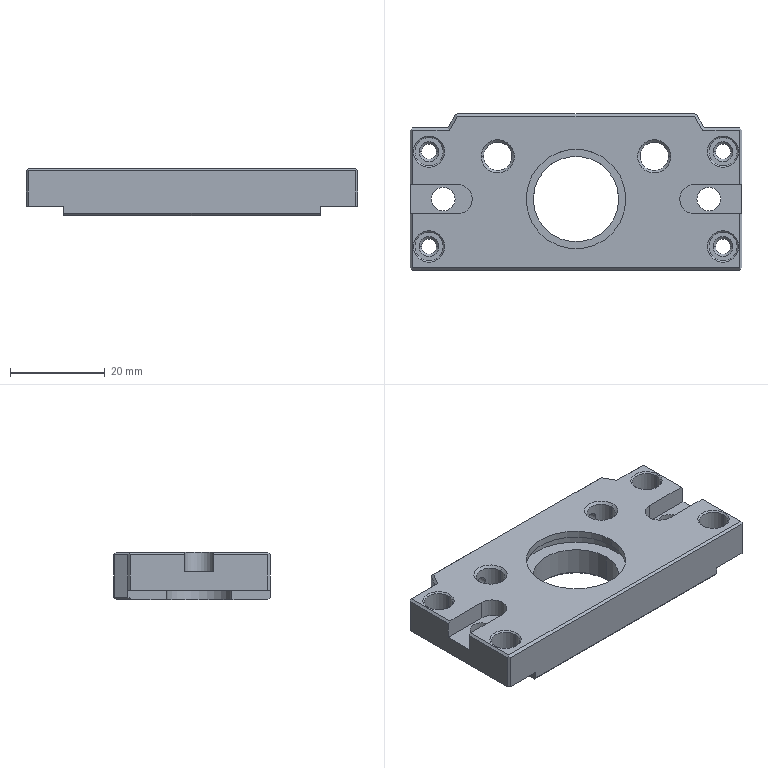NC program | NX | posted with a generic post | part box 70 x 33 x 10 mm
Whole program:
N10 G17 G21 G94 G90
(FACE_MILLING , TOOL : D50面刀)
N12 T01 M6
N14 G54
N16 G17 G0 G90 X62.5 Y0. B0. C0. S4500 M3
N18 G43 Z20. H1
N20 Z3.
N22 G94 G1 Z0. F1000.
N24 X59.5
N26 X-59.5
N28 X-62.5
N30 Z3.
N32 G0 Z20.
N34 M5
(ADAPTIVE_MILLING , TOOL : D8)
N36 T11 M6
N38 G54
N40 G17 G0 G90 X-49.152 Y-2.056 B0. C0. S5500 M3
N42 G43 Z20. H11
N44 Z-8.
N46 G94 G1 Z-11. F1200.
N48 X-47.71 Y-1.981 F2000.
N50 G3 X-47.004 Y-1.481 R0.81
N52 X-46.505 Y1.714 R10.42
N54 X-46.395 Y11.128 R266.832
N56 G1 X-46.37 Y20.877
N58 G2 X-43.682 Y24.459 R4.938
N60 X-38.849 Y25.702 R12.089
N62 X-28.354 Y25.892 R150.349
N64 G1 X41.1 Y25.89
N66 G2 X44.79 Y23.5 R4.704
N68 X46.174 Y18.716 R10.981
N70 X46.392 Y10.321 R101.576
N72 G1 X46.395 Y-20.463
N74 G2 X44.038 Y-24.23 R4.692
N76 X39.179 Y-25.668 R10.952
N78 X30.86 Y-25.89 R98.941
N80 G1 X-40.965 Y-25.893
N82 G2 X-44.663 Y-23.639 R4.657
N84 X-46.149 Y-18.875 R10.553
N86 X-46.392 Y-10.182 R94.46
N88 X-46.345 Y-3.033 R153.115
N90 G3 X-45.8 Y9.035 R101.464
N92 G2 X-45.765 Y18.952 R566.148
N94 X-42.22 Y23.757 R6.189
N96 X-36.715 Y25.09 R14.607
N98 X-25.545 Y25.292 R163.704
N100 G1 X39.075 Y25.289
N102 G2 X44.164 Y21.915 R6.065
N104 X45.582 Y16.359 R14.045
N106 X45.793 Y7.064 R128.382
N108 G1 X45.794 Y-18.363
N110 G2 X42.522 Y-23.585 R6.05
N112 X37.271 Y-25.037 R13.25
N114 X27.902 Y-25.29 R107.811
N116 G1 X-38.865 Y-25.292
N118 G2 X-44.161 Y-21.883 R6.092
N120 X-45.574 Y-16.402 R13.967
N122 X-45.701 Y-3.284 R130.413
N124 G3 X-45.196 Y12.254 R169.82
N126 G2 X-45.128 Y17.675 R70.04
N128 X-40.932 Y23.14 R7.06
N130 X-34.964 Y24.49 R16.783
N132 X-23.493 Y24.692 R178.313
N134 G1 X37.2 Y24.69
N136 G2 X43.615 Y20.499 R7.002
N138 X44.988 Y14.537 R16.528
N140 X45.192 Y5.241 R141.965
N142 G1 X45.194 Y-16.488
N144 G2 X41.022 Y-23.091 R7.038
N146 X35.218 Y-24.469 R16.174
N148 X25.323 Y-24.691 R138.059
N150 G1 X-36.99 Y-24.692
N152 G2 X-43.58 Y-20.541 R7.039
N154 X-44.987 Y-14.515 R16.451
N156 X-44.819 Y0.802 R111.055
N158 G3 X-44.575 Y15.703 R364.89
N160 G2 X-39.873 Y22.491 R7.674
N162 X-33.831 Y23.863 R17.749
N164 X-24.086 Y24.09 R139.103
N166 G1 X35.25 Y24.092
N168 G2 X40.54 Y22.547 R8.089
N170 X43.716 Y17.374 R9.533
N172 X44.517 Y10.461 R30.733
N174 X44.593 Y1.386 R596.65
N176 G1 X44.592 Y-15.064
N178 G2 X39.853 Y-22.496 R7.746
N180 X33.813 Y-23.863 R17.795
N182 X23.843 Y-24.09 R142.789
N184 G1 X-35.34 Y-24.091
N186 G2 X-41.121 Y-22.028 R7.865
N188 X-43.877 Y-16.695 R10.396
N190 X-44.547 Y-9.237 R38.609
N192 X-44.232 Y0.639 R125.315
N194 G3 X-43.968 Y14.506 R422.448
N196 G2 X-38.871 Y21.862 R8.21
N198 X-32.528 Y23.261 R19.053
N200 X-22.483 Y23.489 R147.953
N202 G1 X33.75 Y23.492
N204 G2 X38.493 Y22.603 R10.049
N206 X42.711 Y17.522 R8.884
N208 X43.835 Y10.967 R23.19
N210 X43.993 Y0.019 R238.1
N212 X43.953 Y-14.687 R678.1
N214 X38.901 Y-21.846 R8.196
N216 X32.707 Y-23.245 R18.74
N218 X22.438 Y-23.489 R141.189
N220 G1 X-33.69 Y-23.491
N222 G2 X-38.437 Y-22.62 R10.181
N224 X-42.745 Y-17.406 R8.942
N226 X-43.855 Y-10.545 R24.379
N228 X-43.68 Y-0.337 R99.124
N230 G3 X-43.365 Y13.389 R451.187
N232 G2 X-37.95 Y21.229 R8.658
N234 X-31.236 Y22.666 R20.319
N236 X-18.866 Y22.891 R191.382
N238 G1 X32.775 Y22.889
N240 G2 X37.858 Y21.828 R10.396
N242 X42.114 Y16.487 R9.388
N244 X43.235 Y9.702 R24.845
N246 X43.393 Y-1.471 R251.328
N248 X43.347 Y-13.562 R458.472
N250 X37.861 Y-21.265 R8.657
N252 X31.136 Y-22.673 R20.691
N254 X18.69 Y-22.891 R198.938
N256 G1 X-32.715 Y-22.889
N258 G2 X-37.737 Y-21.882 R10.582
N260 X-42.119 Y-16.449 R9.385
N262 X-43.251 Y-9.137 R25.538
N264 X-43.013 Y1.208 R135.601
N266 G3 X-42.764 Y12.353 R789.434
N268 G2 X-36.952 Y20.652 R9.071
N270 X-30.078 Y22.067 R21.607
N272 X-17.557 Y22.291 R199.457
N274 G1 X31.443 Y22.289
N276 G2 X36.438 Y21.468 R12.236
N278 X41.272 Y16.167 R9.327
N280 X42.575 Y9.495 R22.455
N282 X42.793 Y-3.101 R207.333
N284 X42.737 Y-12.574 R269.883
N286 X37.015 Y-20.622 R9.015
N288 X30.141 Y-22.061 R21.377
N290 X17.545 Y-22.291 R197.541
N292 G1 X-31.38 Y-22.289
N294 G2 X-36.448 Y-21.458 R12.366
N296 X-41.324 Y-16.015 R9.409
N298 X-42.595 Y-8.732 R23.307
N300 X-42.39 Y1.867 R142.482
N302 G1 X-42.165 Y11.389
N304 G2 X-38.994 Y18.274 R9.394
N306 X-32.797 Y20.997 R13.181
N308 X-24.582 Y21.642 R49.89
N310 G1 X-13.633 Y21.691
N312 X30.267 Y21.688
N314 G2 X35.286 Y20.97 R13.86
N316 X40.605 Y15.42 R9.524
N318 X41.956 Y8.678 R22.632
N320 X42.192 Y-3.917 R194.662
N322 X42.107 Y-11.89 R134.653
N324 X37.398 Y-19.4 R9.151
N326 X34.69 Y-20.686 R5.236
N328 X26.055 Y-21.609 R42.604
N330 X13.606 Y-21.691 R670.645
N332 G1 X-31.594 Y-21.676
N334 G2 X-37.656 Y-19.582 R9.918
N336 X-41.195 Y-13.609 R11.252
N338 X-41.995 Y-5.646 R31.702
N340 X-41.68 Y6.09 R866.259
N342 X-41.453 Y11.621 R53.73
N344 X-35.553 Y19.29 R9.539
N346 X-28.627 Y20.816 R21.601
N348 X-17.458 Y21.086 R156.346
N350 G1 X-11.908 Y21.09
N352 X28.825 Y21.089
N354 G2 X33.876 Y20.55 R17.194
N356 X39.855 Y14.906 R9.599
N358 X41.349 Y7.741 R22.558
N360 X41.592 Y-4.929 R193.784
N362 X41.458 Y-11.375 R68.318
N364 X39.02 Y-16.922 R9.611
N366 G1 X38.961 Y-17.059
N368 G3 X39.034 Y-17.505 R0.842
N370 G1 X39.282 Y-18.02
N372 X39.969 Y-19.442 Z-10.9
N374 G2 X39.88 Y-20.491 R0.852
N376 G1 X38.899 Y-21.46
N378 G2 X37.957 Y-21.476 R0.845
N380 G1 X36.537 Y-20.787 Z-11.
N382 X35.906 Y-20.491
N384 G3 X34.498 Y-20.6 R5.077
N386 X28.488 Y-20.893 R94.724
N388 G2 X12.141 Y-21.09 R368.085
N390 G1 X-31.486 Y-21.066
N392 G2 X-33.882 Y-20.6 R20.562
N394 X-36.55 Y-20.051 R5.002
N396 X-39.286 Y-16.648 R7.559
N398 X-41.278 Y-7.923 R22.641
N400 X-41.167 Y2.671 R135.063
N402 X-40.928 Y10.135 R162.022
N404 X-34.607 Y18.738 R9.886
N406 X-27.368 Y20.237 R23.103
N408 G3 X-26.04 Y20.46 R3.147
N410 G1 X-24.978 Y20.6
N412 X25.285 Y20.585
N414 G2 X30.957 Y20.361 R98.573
N416 X39.193 Y14.205 R9.797
N418 X40.72 Y7.119 R22.421
N420 X40.989 Y-4.2 R159.742
N422 X40.833 Y-10.644 R60.182
N424 X39.183 Y-15.334 R12.438
N426 G3 X39.1 Y-16.002 R1.839
N428 G2 X37.898 Y-18.9 R4.404
N430 X35.561 Y-20.46 R5.1
N432 X33.448 Y-20.6 R9.325
N434 G1 X-34.502
N436 G2 X-37.4 Y-19.398 R4.404
N438 X-38.97 Y-16.987 R4.942
N440 X-40.131 Y-11.969 R226.977
N442 X-40.694 Y-2.252 R48.87
N444 X-40.378 Y8.798 R561.554
N446 X-38.996 Y13.819 R12.171
N448 X-37.898 Y15.9 R4.393
N450 X-34.856 Y17.866 R7.824
N452 X-27.923 Y19.53 R25.016
N454 G3 X-27.028 Y20.051 R10.346
N456 G1 X-26.335 Y20.338
N458 G3 X-26.943 Y21.989 R0.88
N460 G1 X-28.446 Y21.505 Z-10.9
N462 X-34.426 Y19.58
N464 X-35.929 Y19.096 Z-11.
N466 X-36.611 Y18.881
N468 X-37.287 Y18.647
N470 G3 X-36.55 Y17.051 R0.88
N472 G2 X-34.662 Y17.607 R5.194
N474 X-28.787 Y18.816 R169.229
N476 G3 X-28.402 Y19.041 R4.343
N478 X-28.361 Y20.214 R0.881
N480 X-29.349 Y20.485 Z-10.931 R0.932
N482 G1 X-29.832 Y20.387 Z-10.9
N484 X-33.835 Y19.577
N486 X-35.383 Y19.264 Z-11.
N488 G3 X-35.189 Y17.509 R-0.883
N490 G2 X-33.066 Y17.627 R16.758
N492 G3 X-29.301 Y18.222 R18.891
N494 X-28.792 Y18.522 R1.747
N496 G2 X-27.657 Y19.651 R3.266
N498 G3 X-27.727 Y21.097 R0.88
N500 X-28.617 Y21.134 Z-10.941 R0.952
N502 G1 X-29.232 Y20.921 Z-10.9
N504 X-33.107 Y19.581
N506 X-34.002 Y19.262 Z-10.96
N508 G3 X-34.416 Y18.806 Z-11. R0.911
N510 X-33.598 Y17.6 R0.88
N512 X-30.105 Y17.672 R28.201
N514 X-28.779 Y18.539 R1.62
N516 X-28.954 Y19.782 R0.88
N518 X-29.966 Y19.821 Z-10.932 R0.935
N520 G1 X-30.429 Y19.617 Z-10.9
N522 X-30.509 Y19.581
N524 X-31.303 Y19.218 Z-10.955
N526 G3 X-31.687 Y18.649 Z-11. R0.905
N528 X-30.823 Y17.6 R0.88
N530 X-29.465 Y17.71 R3.475
N532 X-29.013 Y18.213 R1.248
N534 X-30.443 Y19.226 R0.88
N536 X-30.782 Y18.672 R1.265
N538 X-29.923 Y17.6 R0.88
N540 X-29.167 Y17.964 R0.856
N542 X-29.083 Y18.803 R0.803
N544 X-29.557 Y19.247 Z-10.958 R1.139
N546 G1 X-30.327 Y19.749 Z-10.9
N548 X-31.343 Y20.402
N550 X-31.508 Y20.454
N552 X-31.679 Y20.476
N554 X-32.565 Y20.477
N556 X-33.449 Y20.436
N558 X-34.032 Y20.35
N560 X-34.607 Y20.227
N562 X-36.828 Y19.636
N564 G3 X-39.16 Y18.133 R5.858
N566 X-40.87 Y15.737 R10.691
N568 G1 X-41.128 Y15.165
N570 X-41.351 Y14.578
N572 X-41.792 Y13.256
N574 X-42.185 Y11.92
N576 G3 X-42.728 Y8.363 R20.829
N578 G1 X-42.819 Y6.888
N580 X-42.868 Y5.411
N582 X-43.023 Y-4.947
N584 G3 X-42.663 Y-10.851 R41.445
N586 G1 X-42.377 Y-13.034
N588 X-42.046 Y-15.211
N590 X-41.991 Y-15.397
N592 X-41.897 Y-15.567
N594 X-41.001 Y-16.769
N596 X-40.329 Y-17.657 Z-10.971
N598 G3 X-39.926 Y-17.875 Z-11. R0.854
N600 X-38.97 Y-16.987 R0.8
N602 G2 X-39.174 Y-14.575 R31.249
N604 X-40.07 Y-5.199 R69.975
N606 G1 X-40.058 Y9.898
N608 G3 X-39.105 Y12.181 R35.297
N610 G2 X-38.982 Y13.894 R8.885
N612 G3 X-40.002 Y14.765 R0.8
N614 X-40.529 Y14.309 Z-10.955 R0.921
N616 G1 X-41.005 Y13.589 Z-10.9
N618 X-41.598 Y12.676
N620 X-41.651 Y12.511
N622 X-41.674 Y12.34
N624 X-41.792 Y-13.921
N626 G3 X-41.646 Y-14.385 R0.83
N628 G1 X-41.086 Y-15.18
N630 X-40.47 Y-16.036 Z-10.967
N632 G3 X-40.01 Y-16.267 Z-11. R0.84
N634 X-39.1 Y-15.475 R0.8
N636 X-39.368 Y-7.542 R89.777
N638 G2 X-39.458 Y9.38 R429.218
N640 G1 X-39.1 Y10.478
N642 Y12.278
N644 G3 X-39.968 Y13.076 R0.8
N646 X-40.637 Y12.622 Z-10.947 R0.882
N648 G1 X-41.065 Y12.021 Z-10.9
N650 X-41.709 Y11.097
N652 X-41.77 Y10.915
N654 X-41.792 Y10.724
N656 X-41.29 Y-10.223
N658 X-41.078 Y-11.03
N660 X-40.666 Y-12.554 Z-11.
N662 G3 X-39.1 Y-12.325 R0.8
N664 G1 Y10.55
N666 G3 X-39.461 Y11.219 R0.804
N668 G1 X-39.746 Y11.406
N670 X-41.067 Y12.272 Z-10.9
N672 G2 X-41.516 Y12.682 R1.126
N674 G1 X-41.584 Y12.867
N676 X-41.612 Y13.062
N678 G2 X-41.527 Y14.283 R5.081
N680 X-40.671 Y16.417 R8.617
N682 X-37.461 Y19.173 R6.501
N684 X-28.5 Y22.166 R63.874
N686 X-22.287 Y22.953 R29.2
N688 G1 X-18.342 Y23.005
N690 X-14.397 Y23.033
N692 X22.469 Y23.112
N694 G2 X23.123 Y22.775 R0.805
N696 G1 X23.248 Y22.599
N698 X24.162 Y21.312 Z-11.
N700 X24.518 Y20.829
N702 G3 X24.981 Y20.6 R0.823
N704 G2 X27.322 Y20.176 R24.846
N706 X31.787 Y19.501 R37.364
N708 X35.925 Y17.31 R10.586
N710 X37.4 Y16.398 R4.216
N712 X39.127 Y13.222 R4.939
N714 X40.331 Y1.588 R56.755
N716 X40.299 Y-9.059 R158.783
N718 X39.113 Y-13.848 R16.934
N720 G1 X39.1 Y-15.663
N722 G3 X39.974 Y-16.459 R0.8
N724 X40.639 Y-16.003 Z-10.947 R0.883
N726 G1 X41.065 Y-15.398 Z-10.9
N728 X41.709 Y-14.467
N730 X41.768 Y-14.292
N732 X41.792 Y-14.109
N734 X41.652 Y12.507
N736 G3 X41.52 Y12.944 R0.84
N738 G1 X41.003 Y13.726
N740 X40.34 Y14.709 Z-10.975
N742 X40.189 Y14.832 Z-10.988
N744 X40.015 Y14.921 Z-11.
N746 G3 X38.96 Y14.061 R0.8
N748 G2 X39.112 Y11.402 R13.987
N750 X39.778 Y-4.454 R164.636
N752 X39.403 Y-10.28 R28.17
N754 G1 X39.1 Y-11.595
N756 Y-13.995
N758 G3 X40.654 Y-14.262 R0.8
N760 G1 X41.068 Y-12.739 Z-10.9
N762 X41.29 Y-11.893
N764 X41.792 Y10.169
N766 G3 X41.644 Y10.651 R0.826
N768 G1 X41.088 Y11.433
N770 X40.468 Y12.287 Z-10.967
N772 G3 X40.008 Y12.516 Z-11. R0.84
N774 X39.1 Y11.723 R0.8
N776 X39.163 Y-5.39 R980.797
N778 X39.1 Y-11.656 R133.386
N780 X40.65 Y-11.934 R0.8
N782 G1 X41.068 Y-10.411 Z-10.9
N784 X41.291 Y-9.564
N786 Y-1.319
N788 X41.079 Y-0.515
N790 X40.665 Y1.008 Z-11.
N792 G3 X39.1 Y0.773 R0.8
N794 G1 Y-7.177
N796 G3 X40.456 Y-7.752 R0.8
N798 X40.73 Y-7.235 Z-10.963 R1.238
N800 G1 X41.066 Y-6.307 Z-10.9
N802 X41.344 Y-5.559
N804 X41.6 Y-4.803
N806 X41.612 Y-4.665
N808 Y13.097
N810 G3 X41.16 Y15.493 R7.252
N812 X40.11 Y17.129 R4.047
N814 X38.07 Y18.981 R22.304
N816 X32.307 Y21.91 R18.6
N818 G1 X30.375 Y22.465
N820 X28.436 Y22.996
N822 G3 X27.976 Y22.916 R0.836
N824 G1 X26.778 Y22.313
N826 X26.32 Y22.084 Z-10.932
N828 X25.869 Y21.841 Z-10.965
N830 G3 X25.569 Y21.388 Z-11. R0.836
N832 X26.04 Y20.46 R0.801
N834 X29.78 Y19.339 R16.206
N836 G2 X34.102 Y17.646 R14.998
N838 G1 X35.561 Y17.46
N840 X35.977 Y17.288
N842 G3 X36.572 Y18.942 R-0.88
N844 G1 X36.051 Y19.102
N846 X34.541 Y19.565 Z-10.9
N848 X28.687 Y21.36
N850 X28.14 Y21.53 Z-10.936
N852 X27.588 Y21.684 Z-10.973
N854 X27.373 Y21.683 Z-10.986
N856 X27.163 Y21.636 Z-11.
N858 G3 X27.031 Y20.05 R0.88
N860 X30.236 Y18.669 R14.927
N862 G1 X32.778 Y17.617
N864 X34.393 Y17.6
N866 G3 X35.202 Y18.826 R0.88
N868 X34.515 Y19.364 Z-10.943 R0.959
N870 G1 X33.874 Y19.566 Z-10.9
N872 X29.03 Y21.095
N874 X28.138 Y21.367 Z-10.959
N876 G3 X27.52 Y21.236 Z-11. R0.91
N878 X27.464 Y19.8 R0.88
N880 X31.461 Y17.61 R14.725
N882 G1 X32.96 Y17.6
N884 G3 X33.797 Y18.752 R0.88
N886 X33.107 Y19.361 Z-10.939 R0.956
N888 G1 X32.525 Y19.566 Z-10.9
N890 X29.703 Y20.559
N892 X28.821 Y20.86 Z-10.959
N894 G3 X28.198 Y20.749 Z-11. R0.91
N896 X28.118 Y19.297 R0.88
N898 X29.323 Y18.251 R16.462
N900 X30.578 Y17.6 R3.459
N902 G1 X31.553
N904 G3 X32.423 Y18.609 R0.88
N906 X31.768 Y19.347 Z-10.934 R0.945
N908 G1 X31.276 Y19.565 Z-10.9
N910 X30.089 Y20.091
N912 X29.338 Y20.413 Z-10.952
N914 G3 X28.61 Y20.296 Z-11. R0.896
N916 X28.403 Y19.03 R0.88
N918 X29.831 Y17.645 R4.026
N920 X30.651 Y17.6 R4.966
N922 X31.011 Y19.283 R0.88
N924 G1 X30.4 Y19.562
N926 X29.781 Y19.822
N928 G3 X28.859 Y18.435 R0.88
N930 X29.522 Y17.682 R2.054
N932 X30.076 Y17.6 R2.144
N934 X30.304 Y19.33 R0.88
N936 X29.656 Y19.405 R1.328
N938 X29.076 Y18.104 R0.88
N940 X29.783 Y17.609 R0.864
N942 X30.694 Y18.464 R0.808
N944 G1 X30.619 Y19.573
N946 Z-8.
N948 G0 Z20.
N950 X-3.476 Y-2.422
N952 Z3.
N954 G3 X-3.476 Y-2.422 Z2.605 I3.48 J0.921 F1200.
N956 X-3.476 Y-2.422 Z2.21 I3.48 J0.921
N958 X-3.476 Y-2.422 Z1.816 I3.48 J0.921
N960 X-3.476 Y-2.422 Z1.421 I3.48 J0.921
N962 X-3.476 Y-2.422 Z1.026 I3.48 J0.921
N964 X-3.476 Y-2.422 Z0.631 I3.48 J0.921
N966 X-3.476 Y-2.422 Z0.236 I3.48 J0.921
N968 X-3.476 Y-2.422 Z-0.159 I3.48 J0.921
N970 X-3.476 Y-2.422 Z-0.553 I3.48 J0.921
N972 X-3.476 Y-2.422 Z-0.948 I3.48 J0.921
N974 X-3.476 Y-2.422 Z-1.343 I3.48 J0.921
N976 X-3.476 Y-2.422 Z-1.738 I3.48 J0.921
N978 X-3.476 Y-2.422 Z-2.133 I3.48 J0.921
N980 X-3.476 Y-2.422 Z-2.528 I3.48 J0.921
N982 X-3.476 Y-2.422 Z-2.922 I3.48 J0.921
N984 X-3.476 Y-2.422 Z-3.317 I3.48 J0.921
N986 X-3.476 Y-2.422 Z-3.712 I3.48 J0.921
N988 X-3.476 Y-2.422 Z-4.107 I3.48 J0.921
N990 X-3.476 Y-2.422 Z-4.502 I3.48 J0.921
N992 X-3.476 Y-2.422 Z-4.896 I3.48 J0.921
N994 X-3.476 Y-2.422 Z-5.291 I3.48 J0.921
N996 X-3.476 Y-2.422 Z-5.686 I3.48 J0.921
N998 X-3.476 Y-2.422 Z-6.081 I3.48 J0.921
N1000 X-3.476 Y-2.422 Z-6.476 I3.48 J0.921
N1002 X-3.476 Y-2.422 Z-6.871 I3.48 J0.921
N1004 X-3.476 Y-2.422 Z-7.265 I3.48 J0.921
N1006 X-3.476 Y-2.422 Z-7.66 I3.48 J0.921
N1008 X-3.476 Y-2.422 Z-8.055 I3.48 J0.921
N1010 X-3.476 Y-2.422 Z-8.45 I3.48 J0.921
N1012 X-3.476 Y-2.422 Z-8.845 I3.48 J0.921
N1014 X-3.476 Y-2.422 Z-9.24 I3.48 J0.921
N1016 X-3.476 Y-2.422 Z-9.634 I3.48 J0.921
N1018 X-3.476 Y-2.422 Z-10.029 I3.48 J0.921
N1020 X-3.476 Y-2.422 Z-10.424 I3.48 J0.921
N1022 X-3.476 Y-2.422 Z-10.819 I3.48 J0.921
N1024 X3.604 Y-1.5 Z-11. R3.6
N1026 X-0.119 Y-5.154 R-3.628 F2000.
N1028 X2.445 Y1.501 R3.788
N1030 X2.265 Y-4.718 R-3.906
N1032 X-2.663 Y1.721 R-4.059
N1034 X3.577 Y-3.79 R-4.21
N1036 X-3.08 Y1.736 R4.348
N1038 X3.886 Y-3.869 R-4.506
N1040 X-3.484 Y1.759 R4.654
N1042 X4.178 Y-3.973 R-4.81
N1044 X1.654 Y3.098 R4.848
N1046 X-3.383 Y2.024 R5.024
N1048 X-4.689 Y-2.875 R5.023
N1050 X2.676 Y-5.589 R4.917
N1052 X4.728 Y-2.738 R5.156
N1054 X3.929 Y-1.73 R0.808
N1056 G1 X2.871 Y-1.751
N1058 Z-8.
N1060 G0 Z20.
N1062 M5
(PLANAR_MILL_1 , TOOL : D5精刀)
N1064 T07 M6
N1066 G54
N1068 G17 G0 G90 X-4.5 Y-1.5 B0. C0. S4500 M3
N1070 G43 Z20. H7
N1072 Z-0.7
N1074 G94 G1 Z-3.7 F480.
N1076 X-7.
N1078 G3 X0. Y-8.5 R7. F800.
N1080 X-7. Y-1.5 R-7.
N1082 G1 X-4.5
N1084 X-7.2 F480.
N1086 G3 X0. Y-8.7 R7.2 F800.
N1088 X-7.2 Y-1.5 R-7.2
N1090 G1 X-4.7
N1092 X-7.4 F480.
N1094 G3 X0. Y-8.9 R7.4 F800.
N1096 X-7.4 Y-1.5 R-7.4
N1098 G1 X-4.9
N1100 X-7.6 F480.
N1102 G3 X0. Y-9.1 R7.6 F800.
N1104 X-7.6 Y-1.5 R-7.6
N1106 G1 X-5.1
N1108 X-7.8 F480.
N1110 G3 X0. Y-9.3 R7.8 F800.
N1112 X-7.8 Y-1.5 R-7.8
N1114 G1 X-5.3
N1116 Z-0.7
N1118 G0 Z20.
N1120 M5
(PLANAR_MILL_2_COPY_COPY , TOOL : T_CUTTER)
N1122 T06 M6
N1124 G54
N1126 G17 G0 G90 X-5.603 Y0. B0. C0. S3500 M3
N1128 G43 Z20. H6
N1130 Z-1.1
N1132 G94 G1 Z-3.1 F200.
N1134 X-6.3
N1136 G3 X-7.8 Y-1.5 R1.5
N1138 X0. Y-9.3 R7.8
N1140 X-7.8 Y-1.5 R-7.8
N1142 X-6.3 Y-3. R1.5
N1144 G1 X-5.603
N1146 Z-1.1
N1148 G0 Z20.
(PLANAR_MILL_2 , TOOL : T_CUTTER)
N1150 Y0.
N1152 Z-1.7
N1154 G1 Z-3.7
N1156 X-6.3
N1158 G3 X-7.8 Y-1.5 R1.5
N1160 X0. Y-9.3 R7.8
N1162 X-7.8 Y-1.5 R-7.8
N1164 X-6.3 Y-3. R1.5
N1166 G1 X-5.603
N1168 Z-1.7
N1170 G0 Z20.
(PLANAR_MILL_2_COPY , TOOL : T_CUTTER)
N1172 Y0.
N1174 Z-0.5
N1176 G1 Z-2.5
N1178 X-6.3
N1180 G3 X-7.8 Y-1.5 R1.5
N1182 X0. Y-9.3 R7.8
N1184 X-7.8 Y-1.5 R-7.8
N1186 X-6.3 Y-3. R1.5
N1188 G1 X-5.603
N1190 Z-0.5
N1192 G0 Z20.
N1194 M5
(DRILLING_COPY , TOOL : D10点钻)
N1196 T03 M6
N1198 G54
N1200 G17 G0 G90 X-16.5 Y7.5 B0. C0. S1600 M3
N1202 G43 Z20. H3
N1204 G94 G81 G99 Z-3.5 F200. R2.
N1206 X16.5
N1208 G80
N1210 G0 X16.5 Y7.5 Z20.
(DRILLING_COPY_COPY , TOOL : D10点钻)
N1212 X-28. Y-1.5
N1214 G81 Z-1.5 F200. R2.
N1216 X28.
N1218 G80
N1220 G0 X28. Y-1.5 Z20.
(DRILLING , TOOL : D10点钻)
N1222 X-31. Y8.5
N1224 G81 Z-3.3 F200. R2.
N1226 Y-11.5
N1228 X31. Y8.5
N1230 Y-11.5
N1232 G80
N1234 G0 X31. Y-11.5 Z20.
N1236 M5
(DRILLING_COPY_1 , TOOL : D3.2钻头)
N1238 T04 M6
N1240 G54
N1242 G17 G0 G90 X-31. Y8.5 B0. C0. S1600 M3
N1244 G43 Z20. H4
N1246 G94 G81 G99 Z-11. F200. R2.
N1248 Y-11.5
N1250 X31. Y8.5
N1252 Y-11.5
N1254 G80
N1256 G0 X31. Y-11.5 Z20.
N1258 M5
(DRILLING_2 , TOOL : D5钻头)
N1260 T08 M6
N1262 G54
N1264 G17 G0 G90 X-28. Y-1.5 B0. C0. S1600 M3
N1266 G43 Z20. H8
N1268 G94 G81 G99 Z-11. F250. R3.
N1270 X28.
N1272 G80
N1274 G0 X28. Y-1.5 Z20.
N1276 M5
(PLANAR_MILL , TOOL : D4C)
N1278 T02 M6
N1280 G54
N1282 G17 G0 G90 X-38. Y-2.4 B0. C0. S4500 M3
N1284 G43 Z20. H2
N1286 Z1.025
N1288 G94 G1 Z-0.975 F600.
N1290 X-35.
N1292 X-25. F1000.
N1294 G3 X-24.1 Y-1.5 R0.9
N1296 X-25. Y-0.6 R0.9
N1298 G1 X-35.
N1300 X-38.
N1302 Z1.025
N1304 G0 Z20.
N1306 X38.
N1308 Z1.025
N1310 G1 Z-0.975 F600.
N1312 X35.
N1314 X25. F1000.
N1316 G3 X24.1 Y-1.5 R0.9
N1318 X25. Y-2.4 R0.9
N1320 G1 X35.
N1322 X38.
N1324 Z1.025
N1326 G0 Z20.
N1328 Y-0.6
N1330 Z0.05
N1332 G1 Z-1.95 F600.
N1334 X35.
N1336 X25. F1000.
N1338 G3 X24.1 Y-1.5 R0.9
N1340 X25. Y-2.4 R0.9
N1342 G1 X35.
N1344 X38.
N1346 Z0.05
N1348 G0 Z20.
N1350 X-38.
N1352 Z0.05
N1354 G1 Z-1.95 F600.
N1356 X-35.
N1358 X-25. F1000.
N1360 G3 X-24.1 Y-1.5 R0.9
N1362 X-25. Y-0.6 R0.9
N1364 G1 X-35.
N1366 X-38.
N1368 Z0.05
N1370 G0 Z20.
N1372 Y-2.4
N1374 Z-0.925
N1376 G1 Z-2.925 F600.
N1378 X-35.
N1380 X-25. F1000.
N1382 G3 X-24.1 Y-1.5 R0.9
N1384 X-25. Y-0.6 R0.9
N1386 G1 X-35.
N1388 X-38.
N1390 Z-0.925
N1392 G0 Z20.
N1394 X38.
N1396 Z-0.925
N1398 G1 Z-2.925 F600.
N1400 X35.
N1402 X25. F1000.
N1404 G3 X24.1 Y-1.5 R0.9
N1406 X25. Y-2.4 R0.9
N1408 G1 X35.
N1410 X38.
N1412 Z-0.925
N1414 G0 Z20.
N1416 Y-0.6
N1418 Z-1.9
N1420 G1 Z-3.9 F600.
N1422 X35.
N1424 X25. F1000.
N1426 G3 X24.1 Y-1.5 R0.9
N1428 X25. Y-2.4 R0.9
N1430 G1 X35.
N1432 X38.
N1434 Z-1.9
N1436 G0 Z20.
N1438 X-38.
N1440 Z-1.9
N1442 G1 Z-3.9 F600.
N1444 X-35.
N1446 X-25. F1000.
N1448 G3 X-24.1 Y-1.5 R0.9
N1450 X-25. Y-0.6 R0.9
N1452 G1 X-35.
N1454 X-38.
N1456 Z-1.9
N1458 G0 Z20.
(HOLE_MILLING_COPY , TOOL : D4C)
N1460 X-16.5 Y7.5
N1462 Z0.2
N1464 G3 X-16.075 Y7.075 R0.425 F200.
N1466 X-15.65 Y7.5 R0.425
N1468 X-15.65 Y7.5 Z-0.3 I-0.85 J0.
N1470 X-15.65 Y7.5 Z-0.8 I-0.85 J0.
N1472 X-15.65 Y7.5 Z-1.3 I-0.85 J0.
N1474 X-15.65 Y7.5 Z-1.8 I-0.85 J0.
N1476 X-15.65 Y7.5 Z-2.3 I-0.85 J0.
N1478 X-15.65 Y7.5 Z-2.8 I-0.85 J0.
N1480 X-15.65 Y7.5 Z-3.3 I-0.85 J0.
N1482 X-15.65 Y7.5 Z-3.8 I-0.85 J0.
N1484 X-15.65 Y7.5 Z-4.3 I-0.85 J0.
N1486 X-15.65 Y7.5 Z-4.8 I-0.85 J0.
N1488 X-15.65 Y7.5 Z-5.3 I-0.85 J0.
N1490 X-15.65 Y7.5 Z-5.8 I-0.85 J0.
N1492 X-15.65 Y7.5 Z-6.3 I-0.85 J0.
N1494 X-15.65 Y7.5 Z-6.8 I-0.85 J0.
N1496 X-15.65 Y7.5 Z-7.3 I-0.85 J0.
N1498 X-15.65 Y7.5 Z-7.8 I-0.85 J0.
N1500 X-15.65 Y7.5 Z-8.3 I-0.85 J0.
N1502 X-15.65 Y7.5 Z-8.8 I-0.85 J0.
N1504 X-15.65 Y7.5 Z-9.3 I-0.85 J0.
N1506 X-15.65 Y7.5 Z-9.8 I-0.85 J0.
N1508 X-17.188 Y8. Z-10. R0.85
N1510 X-17. Y6.812 R0.85
N1512 X-17.188 Y8. R-0.85
N1514 X-17.094 Y7.406 R0.425
N1516 X-16.5 Y7.5 R0.425
N1518 G0 Z20.
N1520 X16.5
N1522 Z0.2
N1524 G3 X16.925 Y7.075 R0.425
N1526 X17.35 Y7.5 R0.425
N1528 X17.35 Y7.5 Z-0.3 I-0.85 J0.
N1530 X17.35 Y7.5 Z-0.8 I-0.85 J0.
N1532 X17.35 Y7.5 Z-1.3 I-0.85 J0.
N1534 X17.35 Y7.5 Z-1.8 I-0.85 J0.
N1536 X17.35 Y7.5 Z-2.3 I-0.85 J0.
N1538 X17.35 Y7.5 Z-2.8 I-0.85 J0.
N1540 X17.35 Y7.5 Z-3.3 I-0.85 J0.
N1542 X17.35 Y7.5 Z-3.8 I-0.85 J0.
N1544 X17.35 Y7.5 Z-4.3 I-0.85 J0.
N1546 X17.35 Y7.5 Z-4.8 I-0.85 J0.
N1548 X17.35 Y7.5 Z-5.3 I-0.85 J0.
N1550 X17.35 Y7.5 Z-5.8 I-0.85 J0.
N1552 X17.35 Y7.5 Z-6.3 I-0.85 J0.
N1554 X17.35 Y7.5 Z-6.8 I-0.85 J0.
N1556 X17.35 Y7.5 Z-7.3 I-0.85 J0.
N1558 X17.35 Y7.5 Z-7.8 I-0.85 J0.
N1560 X17.35 Y7.5 Z-8.3 I-0.85 J0.
N1562 X17.35 Y7.5 Z-8.8 I-0.85 J0.
N1564 X17.35 Y7.5 Z-9.3 I-0.85 J0.
N1566 X17.35 Y7.5 Z-9.8 I-0.85 J0.
N1568 X15.812 Y8. Z-10. R0.85
N1570 X16. Y6.812 R0.85
N1572 X15.812 Y8. R-0.85
N1574 X15.906 Y7.406 R0.425
N1576 X16.5 Y7.5 R0.425
N1578 G0 Z20.
(DRILLING_COPY_2 , TOOL : D5倒角刀)
N1580 T05 M6
N1582 G17 G43 G0 G90 X-31. Y8.5 Z20. B0. C0. S1600 H5 M3
N1584 G94 G81 G99 Z-7.1 F200. R1.
N1586 Y-11.5
N1588 X31. Y8.5
N1590 Y-11.5
N1592 G80
N1594 G0 X31. Y-11.5 Z20.
(PLANAR_MILL_1_COPY_COPY , TOOL : D5倒角刀)
N1596 X-8.15 Y-0.5 S4500
N1598 Z-0.5
N1600 G1 Z-1.5 F480.
N1602 G3 X-9.15 Y-1.5 R1.
N1604 X0. Y-10.65 R9.15 F800.
N1606 X-9.15 Y-1.5 R-9.15
N1608 X-8.15 Y-2.5 R1.
N1610 G1 Z-0.5
N1612 G0 Z20.
(PLANAR_MILL_1_COPY_COPY_COPY , TOOL : D5倒角刀)
N1614 X-6.15 Y-0.5
N1616 Z-4.7
N1618 G1 Z-5.7 F480.
N1620 G3 X-7.15 Y-1.5 R1.
N1622 X0. Y-8.65 R7.15 F800.
N1624 X-7.15 Y-1.5 R-7.15
N1626 X-6.15 Y-2.5 R1.
N1628 G1 Z-4.7
N1630 G0 Z20.
(PLANAR_MILL_1_COPY , TOOL : D5精刀)
N1632 T07 M6
N1634 G17 G43 G0 G90 X-6.808 Y-0.535 Z20. B0. C0. S4500 H7 M3
N1636 Z-2.7
N1638 G94 G1 Z-3.7 F400.
N1640 G41 X-7.005 Y-0.5 D7
N1642 G3 X-8.005 Y-1.5 R1.
N1644 X0. Y-9.505 R8.005
N1646 X-8.005 Y-1.5 R-8.005
N1648 X-7.005 Y-2.5 R1.
N1650 G40
N1652 G1 X-6.808 Y-2.465
N1654 Z-2.7
N1656 G0 Z20.
(PLANAR_PROFILE_COPY , TOOL : D5精刀)
N1658 X3.834 Y-3.465
N1660 Z-9.
N1662 G1 Z-11.
N1664 G41 X4.031 Y-3.5
N1666 X4.5
N1668 G3 X6.5 Y-1.5 R2.
N1670 X0. Y5. R6.5
N1672 X6.5 Y-1.5 R-6.5
N1674 X4.5 Y0.5 R2.
N1676 G1 X4.031
N1678 G40
N1680 X3.834 Y0.465
N1682 Z-9.
N1684 G0 Z20.
(FACE_MILLING_1 , TOOL : D50面刀)
N1686 T01 M6
N1688 G17 G43 G0 G90 X-84.5 Y0. Z20. B0. C0. S3500 H1 M3
N1690 Z6.025
N1692 G94 G1 Z3.025 F1000.
N1694 X-59.5
N1696 X59.5
N1698 X84.5
N1700 Z6.025
N1702 G0 Z20.
N1704 X-84.5
N1706 Z5.05
N1708 G1 Z2.05
N1710 X-59.5
N1712 X59.5
N1714 X84.5
N1716 Z5.05
N1718 G0 Z20.
N1720 X-84.5
N1722 Z4.075
N1724 G1 Z1.075
N1726 X-59.5
N1728 X59.5
N1730 X84.5
N1732 Z4.075
N1734 G0 Z20.
N1736 X-84.5
N1738 Z3.1
N1740 G1 Z0.1
N1742 X-59.5
N1744 X59.5
N1746 X84.5
N1748 Z3.1
N1750 G0 Z20.
(FACE_MILLING_1_COPY , TOOL : D50面刀)
N1752 X-84.5
N1754 Z3.
N1756 G1 Z0. F600.
N1758 X-59.5
N1760 X59.5
N1762 X84.5
N1764 Z3.
N1766 G0 Z20.
N1768 M5
(FACE_MILLING_2 , TOOL : D5精刀)
N1770 T07 M6
N1772 G54
N1774 G17 G0 G90 X-36.83 Y-21.241 B0. C0. S4500 M3
N1776 G43 Z20. H7
N1778 Z2.05
N1780 G94 G1 Z-0.95 F600.
N1782 X-37.163 Y-17.373
N1784 G2 X-37.2 Y-16.5 R10.2 F1000.
N1786 G1 Y-8.428
N1788 G2 X-34.486 Y-1.5 R10.2
N1790 X-37.2 Y5.428 R10.2
N1792 G1 Y13.5
N1794 G2 X-37.163 Y14.373 R10.2
N1796 G1 X-36.83 Y18.241
N1798 Z2.05
N1800 G0 Z20.
N1802 X-31.895 Y-21.5
N1804 Z2.05
N1806 G1 Z-0.95 F600.
N1808 X-32.946 Y-19.
N1810 G2 X-33.45 Y-16.5 R6.45 F1000.
N1812 G1 Y-8.428
N1814 G2 X-27.921 Y-2.044 R6.45
N1816 G3 X-27.921 Y-0.956 R0.55
N1818 G2 X-33.45 Y5.428 R6.45
N1820 G1 Y13.5
N1822 G2 X-32.946 Y16. R6.45
N1824 G1 X-31.895 Y18.5
N1826 Z2.05
N1828 G0 Z20.
N1830 X-21.401 Y-21.7
N1832 Z2.05
N1834 G1 Z-0.95 F600.
N1836 X-28.02 Y-19.
N1838 G2 X-29.7 Y-16.5 R2.7 F1000.
N1840 G1 Y-8.428
N1842 G2 X-27.386 Y-5.756 R2.7
N1844 G3 X-27.386 Y2.756 R4.3
N1846 G2 X-29.7 Y5.428 R2.7
N1848 G1 Y13.5
N1850 G2 X-29.338 Y14.85 R2.7
N1852 G1 X-28.674 Y16.
N1854 X-25.393 Y21.684
N1856 Z2.05
N1858 G0 Z20.
N1860 X-36.83 Y-21.241
N1862 Z1.1
N1864 G1 Z-1.9 F600.
N1866 X-37.163 Y-17.373
N1868 G2 X-37.2 Y-16.5 R10.2 F1000.
N1870 G1 Y-8.428
N1872 G2 X-34.486 Y-1.5 R10.2
N1874 X-37.2 Y5.428 R10.2
N1876 G1 Y13.5
N1878 G2 X-37.163 Y14.373 R10.2
N1880 G1 X-36.83 Y18.241
N1882 Z1.1
N1884 G0 Z20.
N1886 X-31.895 Y-21.5
N1888 Z1.1
N1890 G1 Z-1.9 F600.
N1892 X-32.946 Y-19.
N1894 G2 X-33.45 Y-16.5 R6.45 F1000.
N1896 G1 Y-8.428
N1898 G2 X-27.921 Y-2.044 R6.45
N1900 G3 X-27.921 Y-0.956 R0.55
N1902 G2 X-33.45 Y5.428 R6.45
N1904 G1 Y13.5
N1906 G2 X-32.946 Y16. R6.45
N1908 G1 X-31.895 Y18.5
N1910 Z1.1
N1912 G0 Z20.
N1914 X-21.401 Y-21.7
N1916 Z1.1
N1918 G1 Z-1.9 F600.
N1920 X-28.02 Y-19.
N1922 G2 X-29.7 Y-16.5 R2.7 F1000.
N1924 G1 Y-8.428
N1926 G2 X-27.386 Y-5.756 R2.7
N1928 G3 X-27.386 Y2.756 R4.3
N1930 G2 X-29.7 Y5.428 R2.7
N1932 G1 Y13.5
N1934 G2 X-29.338 Y14.85 R2.7
N1936 G1 X-28.674 Y16.
N1938 X-25.393 Y21.684
N1940 Z1.1
N1942 G0 Z20.
N1944 X36.83 Y18.241
N1946 Z2.05
N1948 G1 Z-0.95 F600.
N1950 X37.163 Y14.373
N1952 G2 X37.2 Y13.5 R10.2 F1000.
N1954 G1 Y5.428
N1956 G2 X34.486 Y-1.5 R10.2
N1958 X37.2 Y-8.428 R10.2
N1960 G1 Y-16.5
N1962 G2 X37.163 Y-17.373 R10.2
N1964 G1 X36.83 Y-21.241
N1966 Z2.05
N1968 G0 Z20.
N1970 X31.895 Y18.5
N1972 Z2.05
N1974 G1 Z-0.95 F600.
N1976 X32.946 Y16.
N1978 G2 X33.45 Y13.5 R6.45 F1000.
N1980 G1 Y5.428
N1982 G2 X27.921 Y-0.956 R6.45
N1984 G3 X27.921 Y-2.044 R0.55
N1986 G2 X33.45 Y-8.428 R6.45
N1988 G1 Y-16.5
N1990 G2 X32.946 Y-19. R6.45
N1992 G1 X31.895 Y-21.5
N1994 Z2.05
N1996 G0 Z20.
N1998 X25.393 Y21.684
N2000 Z2.05
N2002 G1 Z-0.95 F600.
N2004 X28.674 Y16.
N2006 X29.338 Y14.85 F1000.
N2008 G2 X29.7 Y13.5 R2.7
N2010 G1 Y5.428
N2012 G2 X27.386 Y2.756 R2.7
N2014 G3 X27.386 Y-5.756 R4.3
N2016 G2 X29.7 Y-8.428 R2.7
N2018 G1 Y-16.5
N2020 G2 X28.02 Y-19. R2.7
N2022 G1 X21.401 Y-21.7
N2024 Z2.05
N2026 G0 Z20.
N2028 X36.83 Y18.241
N2030 Z1.1
N2032 G1 Z-1.9 F600.
N2034 X37.163 Y14.373
N2036 G2 X37.2 Y13.5 R10.2 F1000.
N2038 G1 Y5.428
N2040 G2 X34.486 Y-1.5 R10.2
N2042 X37.2 Y-8.428 R10.2
N2044 G1 Y-16.5
N2046 G2 X37.163 Y-17.373 R10.2
N2048 G1 X36.83 Y-21.241
N2050 Z1.1
N2052 G0 Z20.
N2054 X31.895 Y18.5
N2056 Z1.1
N2058 G1 Z-1.9 F600.
N2060 X32.946 Y16.
N2062 G2 X33.45 Y13.5 R6.45 F1000.
N2064 G1 Y5.428
N2066 G2 X27.921 Y-0.956 R6.45
N2068 G3 X27.921 Y-2.044 R0.55
N2070 G2 X33.45 Y-8.428 R6.45
N2072 G1 Y-16.5
N2074 G2 X32.946 Y-19. R6.45
N2076 G1 X31.895 Y-21.5
N2078 Z1.1
N2080 G0 Z20.
N2082 X25.393 Y21.684
N2084 Z1.1
N2086 G1 Z-1.9 F600.
N2088 X28.674 Y16.
N2090 X29.338 Y14.85 F1000.
N2092 G2 X29.7 Y13.5 R2.7
N2094 G1 Y5.428
N2096 G2 X27.386 Y2.756 R2.7
N2098 G3 X27.386 Y-5.756 R4.3
N2100 G2 X29.7 Y-8.428 R2.7
N2102 G1 Y-16.5
N2104 G2 X28.02 Y-19. R2.7
N2106 G1 X21.401 Y-21.7
N2108 Z1.1
N2110 G0 Z20.
N2112 M5
(PLANAR_PROFILE_2_COPY_COPY , TOOL : D5倒角刀)
N2114 T05 M6
N2116 G54
N2118 G17 G0 G90 X-4.33 Y1. B0. C0. S4500 M3
N2120 G43 Z20. H5
N2122 Z1.5
N2124 G94 G1 Z-1.5 F1000.
N2126 X-5.5
N2128 G3 X-8. Y-1.5 R2.5
N2130 X0. Y-9.5 R8.
N2132 X-8. Y-1.5 R-8.
N2134 X-5.5 Y-4. R2.5
N2136 G1 X-4.33
N2138 Z1.5
N2140 G0 Z20.
(PLANAR_PROFILE_2_COPY_COPY_COPY , TOOL : D5倒角刀)
N2142 X-17.914 Y8.
N2144 Z-0.5
N2146 G1 Z-1.5
N2148 X-18.
N2150 G3 X-18.5 Y7.5 R0.5
N2152 X-16.5 Y5.5 R2.
N2154 X-18.5 Y7.5 R-2.
N2156 X-18. Y7. R0.5
N2158 G1 X-17.914
N2160 Z-0.5
N2162 G0 Z20.
N2164 X17. Y8.914
N2166 Z-0.5
N2168 G1 Z-1.5
N2170 Y9.
N2172 G3 X16.5 Y9.5 R0.5
N2174 X14.5 Y7.5 R2.
N2176 X16.5 Y9.5 R-2.
N2178 X16. Y9. R0.5
N2180 G1 Y8.914
N2182 Z-0.5
N2184 G0 Z20.
N2186 M5
(FACE_MILLING_2_COPY , TOOL : D5精刀)
N2188 T07 M6
N2190 G54
N2192 G17 G0 G90 X-36.528 Y-21.5 B0. C0. S4500 M3
N2194 G43 Z20. H7
N2196 Z1.
N2198 G94 G1 Z-2. F600.
N2200 X-36.945 Y-17.548
N2202 G2 X-37. Y-16.5 R10.
N2204 G1 Y-8.428
N2206 G2 X-34.211 Y-1.5 R10.
N2208 X-37. Y5.428 R10.
N2210 G1 Y13.5
N2212 G2 X-36.945 Y14.548 R10.
N2214 G1 X-36.528 Y18.5
N2216 Z1.
N2218 G0 Z20.
N2220 X-31.653 Y-21.5
N2222 Z1.
N2224 G1 Z-2.
N2226 X-32.741 Y-18.97
N2228 G2 X-33.25 Y-16.5 R6.25
N2230 G1 Y-8.428
N2232 G2 X-27.893 Y-2.242 R6.25
N2234 G3 X-27.893 Y-0.758 R0.75
N2236 G2 X-33.25 Y5.428 R6.25
N2238 G1 Y13.5
N2240 G2 X-32.741 Y15.97 R6.25
N2242 G1 X-31.653 Y18.5
N2244 Z1.
N2246 G0 Z20.
N2248 X-24.916 Y-21.5
N2250 Z1.
N2252 G1 Z-2.
N2254 Y-19.356
N2256 X-27.386 Y-18.97
N2258 G2 X-29.5 Y-16.5 R2.5
N2260 G1 Y-8.428
N2262 G2 X-27.357 Y-5.954 R2.5
N2264 G3 X-27.357 Y2.954 R4.5
N2266 G2 X-29.5 Y5.428 R2.5
N2268 G1 Y13.5
N2270 G2 X-29.165 Y14.75 R2.5
N2272 G1 X-28.461 Y15.97
N2274 X-25.273 Y21.491
N2276 Z1.
N2278 G0 Z20.
N2280 X36.528 Y18.5
N2282 Z1.
N2284 G1 Z-2.
N2286 X36.945 Y14.548
N2288 G2 X37. Y13.5 R10.
N2290 G1 Y5.428
N2292 G2 X34.211 Y-1.5 R10.
N2294 X37. Y-8.428 R10.
N2296 G1 Y-16.5
N2298 G2 X36.945 Y-17.548 R10.
N2300 G1 X36.528 Y-21.5
N2302 Z1.
N2304 G0 Z20.
N2306 X31.653 Y18.5
N2308 Z1.
N2310 G1 Z-2.
N2312 X32.741 Y15.97
N2314 G2 X33.25 Y13.5 R6.25
N2316 G1 Y5.428
N2318 G2 X27.893 Y-0.758 R6.25
N2320 G3 X27.893 Y-2.242 R0.75
N2322 G2 X33.25 Y-8.428 R6.25
N2324 G1 Y-16.5
N2326 G2 X32.741 Y-18.97 R6.25
N2328 G1 X31.653 Y-21.5
N2330 Z1.
N2332 G0 Z20.
N2334 X25.273 Y21.491
N2336 Z1.
N2338 G1 Z-2.
N2340 X28.461 Y15.97
N2342 X29.165 Y14.75
N2344 G2 X29.5 Y13.5 R2.5
N2346 G1 Y5.428
N2348 G2 X27.357 Y2.954 R2.5
N2350 G3 X27.357 Y-5.954 R4.5
N2352 G2 X29.5 Y-8.428 R2.5
N2354 G1 Y-16.5
N2356 G2 X27.386 Y-18.97 R2.5
N2358 G1 X24.916 Y-19.356
N2360 Y-21.5
N2362 Z1.
N2364 G0 Z20.
(HOLE_MILLING_1 , TOOL : D5精刀)
N2366 X-16.5 Y7.5
N2368 Z-10.
N2370 G41 G1 X-16.523 Y7.597 F200. D7
N2372 G3 X-17. Y7.5 R0.249
N2374 X-16.5 Y7. R0.5
N2376 X-17. Y7.5 R-0.5
N2378 X-16.523 Y7.403 R0.249
N2380 G40
N2382 G1 X-16.5 Y7.5
N2384 G0 Z20.
N2386 X16.5
N2388 Z-10.
N2390 G41 G1 X16.477 Y7.597
N2392 G3 X16. Y7.5 R0.249
N2394 X16.5 Y7. R0.5
N2396 X16. Y7.5 R-0.5
N2398 X16.477 Y7.403 R0.249
N2400 G40
N2402 G1 X16.5 Y7.5
N2404 G0 Z20.
N2406 M5
(DRILLING_1 , TOOL : D5倒角刀)
N2408 T05 M6
N2410 G54
N2412 G17 G0 G90 X-23. Y0. B0. C0. S2000 M3
N2414 G43 Z20. H5
N2416 G94 G81 G99 Z-1.7 F200. R3.
N2418 X-16.5 Y-1.5
N2420 X16.5
N2422 X23. Y0.
N2424 G80
N2426 G0 X23. Y0. Z20.
N2428 M5
(DRILLING_1_COPY , TOOL : D2.6)
N2430 T09 M6
N2432 G54
N2434 G17 G0 G90 X-23. Y0. B0. C0. S3000 M3
N2436 G43 Z20. H9
N2438 G94 G81 G99 Z-10.5 F200. R3.
N2440 X-16.5 Y-1.5
N2442 X16.5
N2444 X23. Y0.
N2446 G80
N2448 G0 X23. Y0. Z20.
N2450 M5
(DRILLING_1_COPY_COPY , TOOL : M3)
N2452 T10 M6
N2454 G54
N2456 G17 G0 G90 X-23. Y0. B0. C0. S300 M3
N2458 G43 Z20. H10
N2460 G94 G81 G99 Z-6. R3.
N2462 X-16.5 Y-1.5
N2464 X16.5
N2466 X23. Y0.
N2468 G80
N2470 G0 X23. Y0. Z20.
N2472 M5
(ZLEVEL_PROFILE , TOOL : D5精刀)
N2474 T07 M6
N2476 G54
N2478 G17 G0 G90 X27.531 Y8.272 B0. C0. S5500 M3
N2480 G43 Z20. H7
N2482 Z0.97
N2484 G94 G1 Z-0.03 F1500.
N2486 Y4.53
N2488 Y-4.53
N2490 X27.583 Y-4.56 Z-0.06
N2492 Y4.56
N2494 X27.635 Y4.59 Z-0.09
N2496 Y-4.59
N2498 X27.687 Y-4.609 Z-0.12
N2500 Y4.609
N2502 X27.739 Y4.6 Z-0.15
N2504 Y-4.6
N2506 X27.791 Y-4.57 Z-0.18
N2508 Y4.57
N2510 X27.843 Y4.54 Z-0.21
N2512 Y-4.54
N2514 X27.895 Y-4.51 Z-0.24
N2516 Y4.51
N2518 X27.924 Y4.5 Z-0.27
N2520 Y-4.5
N2522 X27.941 Z-0.3
N2524 Y4.5
N2526 X27.958 Z-0.33
N2528 Y-4.5
N2530 X27.976 Z-0.36
N2532 Y4.5
N2534 X27.993 Z-0.39
N2536 Y-4.5
N2538 X28.01 Z-0.42
N2540 Y4.5
N2542 X28.028 Z-0.45
N2544 Y-4.5
N2546 X28.045 Z-0.48
N2548 Y4.5
N2550 X28.062 Z-0.51
N2552 Y-4.5
N2554 X28.08 Z-0.54
N2556 Y4.5
N2558 X28.097 Z-0.57
N2560 Y-4.5
N2562 X28.114 Z-0.6
N2564 Y4.5
N2566 X28.132 Z-0.63
N2568 Y-4.5
N2570 X28.149 Z-0.66
N2572 Y4.5
N2574 X28.166 Z-0.69
N2576 Y-4.5
N2578 X28.184 Z-0.72
N2580 Y4.5
N2582 X28.201 Z-0.75
N2584 Y-4.5
N2586 X28.218 Z-0.78
N2588 Y4.5
N2590 X28.236 Z-0.81
N2592 Y-4.5
N2594 X28.253 Z-0.84
N2596 Y4.5
N2598 X28.27 Z-0.87
N2600 Y-4.5
N2602 X28.288 Z-0.9
N2604 Y4.5
N2606 X28.305 Z-0.93
N2608 Y-4.5
N2610 X28.322 Z-0.96
N2612 Y4.5
N2614 X28.34 Z-0.99
N2616 Y-4.5
N2618 X28.357 Z-1.02
N2620 Y4.5
N2622 X28.374 Z-1.05
N2624 Y-4.5
N2626 X28.391 Z-1.08
N2628 Y4.5
N2630 X28.409 Z-1.11
N2632 Y-4.5
N2634 X28.426 Z-1.14
N2636 Y4.5
N2638 X28.443 Z-1.17
N2640 Y-4.5
N2642 X28.461 Z-1.2
N2644 Y4.5
N2646 X28.478 Z-1.23
N2648 Y-4.5
N2650 X28.495 Z-1.26
N2652 Y4.5
N2654 X28.513 Z-1.29
N2656 Y-4.5
N2658 X28.53 Z-1.32
N2660 Y4.5
N2662 X28.547 Z-1.35
N2664 Y-4.5
N2666 X28.565 Z-1.38
N2668 Y4.5
N2670 X28.582 Z-1.41
N2672 Y-4.5
N2674 X28.599 Z-1.44
N2676 Y4.5
N2678 X28.617 Z-1.47
N2680 Y-4.5
N2682 X28.634 Z-1.5
N2684 Y4.5
N2686 X28.651 Z-1.53
N2688 Y-4.5
N2690 X28.669 Z-1.56
N2692 Y4.5
N2694 X28.686 Z-1.59
N2696 Y-4.5
N2698 X28.703 Z-1.62
N2700 Y4.5
N2702 X28.721 Z-1.65
N2704 Y-4.5
N2706 X28.738 Z-1.68
N2708 Y4.5
N2710 X28.755 Z-1.71
N2712 Y-4.5
N2714 X28.773 Z-1.74
N2716 Y4.5
N2718 X28.79 Z-1.77
N2720 Y-4.5
N2722 X28.807 Z-1.8
N2724 Y4.5
N2726 X28.825 Z-1.83
N2728 Y-4.5
N2730 X28.842 Z-1.86
N2732 Y4.5
N2734 X28.859 Z-1.89
N2736 Y-4.5
N2738 X28.876 Z-1.92
N2740 Y4.5
N2742 X28.894 Z-1.95
N2744 Y-4.5
N2746 X28.911 Z-1.98
N2748 Y4.5
N2750 X28.928 Z-2.01
N2752 Y-4.5
N2754 X28.946 Z-2.04
N2756 Y4.5
N2758 X28.963 Z-2.07
N2760 Y-4.5
N2762 X28.98 Z-2.1
N2764 Y4.5
N2766 X28.998 Z-2.13
N2768 Y-4.5
N2770 X29.015 Z-2.16
N2772 Y4.5
N2774 X29.032 Z-2.19
N2776 Y-4.5
N2778 X29.05 Z-2.22
N2780 Y4.5
N2782 X29.067 Z-2.25
N2784 Y-4.5
N2786 X29.084 Z-2.28
N2788 Y4.5
N2790 X29.102 Z-2.31
N2792 Y-4.5
N2794 X29.119 Z-2.34
N2796 Y4.5
N2798 X29.136 Z-2.37
N2800 Y-4.5
N2802 X29.154 Z-2.4
N2804 Y4.5
N2806 X29.171 Z-2.43
N2808 Y-4.5
N2810 X29.188 Z-2.46
N2812 Y4.5
N2814 X29.206 Z-2.49
N2816 Y-4.5
N2818 X29.223 Z-2.52
N2820 Y4.5
N2822 X29.24 Z-2.55
N2824 Y-4.5
N2826 X29.258 Z-2.58
N2828 Y4.5
N2830 X29.275 Z-2.61
N2832 Y-4.5
N2834 X29.292 Z-2.64
N2836 Y4.5
N2838 X29.309 Z-2.67
N2840 Y-4.5
N2842 X29.327 Z-2.7
N2844 Y4.5
N2846 X29.344 Z-2.73
N2848 Y-4.5
N2850 X29.361 Z-2.76
N2852 Y4.5
N2854 X29.379 Z-2.79
N2856 Y-4.5
N2858 X29.396 Z-2.82
N2860 Y4.5
N2862 X29.413 Z-2.85
N2864 Y-4.5
N2866 X29.431 Z-2.88
N2868 Y4.5
N2870 X29.448 Z-2.91
N2872 Y-4.5
N2874 X29.465 Z-2.94
N2876 Y4.5
N2878 X29.483 Z-2.97
N2880 Y-4.5
N2882 X29.491 Z-2.985
N2884 X29.5 Z-3.
N2886 Y4.5
N2888 Y8.288
N2890 Z-2.
N2892 G0 Z20.
N2894 X-27.531 Y-8.272
N2896 Z0.97
N2898 G1 Z-0.03
N2900 Y-4.53
N2902 Y4.53
N2904 X-27.583 Y4.56 Z-0.06
N2906 Y-4.56
N2908 X-27.635 Y-4.59 Z-0.09
N2910 Y4.59
N2912 X-27.687 Y4.609 Z-0.12
N2914 Y-4.609
N2916 X-27.739 Y-4.6 Z-0.15
N2918 Y4.579
N2920 X-27.791 Y4.57 Z-0.18
N2922 Y-4.57
N2924 X-27.843 Y-4.54 Z-0.21
N2926 Y4.54
N2928 X-27.895 Y4.51 Z-0.24
N2930 Y-4.51
N2932 X-27.924 Y-4.5 Z-0.27
N2934 Y4.5
N2936 X-27.941 Z-0.3
N2938 Y-4.5
N2940 X-27.958 Z-0.33
N2942 Y4.5
N2944 X-27.976 Z-0.36
N2946 Y-4.5
N2948 X-27.993 Z-0.39
N2950 Y4.5
N2952 X-28.01 Z-0.42
N2954 Y-4.5
N2956 X-28.028 Z-0.45
N2958 Y4.5
N2960 X-28.045 Z-0.48
N2962 Y-4.5
N2964 X-28.062 Z-0.51
N2966 Y4.5
N2968 X-28.08 Z-0.54
N2970 Y-4.5
N2972 X-28.097 Z-0.57
N2974 Y4.5
N2976 X-28.114 Z-0.6
N2978 Y-4.5
N2980 X-28.132 Z-0.63
N2982 Y4.5
N2984 X-28.149 Z-0.66
N2986 Y-4.5
N2988 X-28.166 Z-0.69
N2990 Y4.5
N2992 X-28.184 Z-0.72
N2994 Y-4.5
N2996 X-28.201 Z-0.75
N2998 Y4.5
N3000 X-28.218 Z-0.78
N3002 Y-4.5
N3004 X-28.236 Z-0.81
N3006 Y4.5
N3008 X-28.253 Z-0.84
N3010 Y-4.5
N3012 X-28.27 Z-0.87
N3014 Y4.5
N3016 X-28.288 Z-0.9
N3018 Y-4.5
N3020 X-28.305 Z-0.93
N3022 Y4.5
N3024 X-28.322 Z-0.96
N3026 Y-4.5
N3028 X-28.34 Z-0.99
N3030 Y4.5
N3032 X-28.357 Z-1.02
N3034 Y-4.5
N3036 X-28.374 Z-1.05
N3038 Y4.5
N3040 X-28.391 Z-1.08
N3042 Y-4.5
N3044 X-28.409 Z-1.11
N3046 Y4.5
N3048 X-28.426 Z-1.14
N3050 Y-4.5
N3052 X-28.443 Z-1.17
N3054 Y4.5
N3056 X-28.461 Z-1.2
N3058 Y-4.5
N3060 X-28.478 Z-1.23
N3062 Y4.5
N3064 X-28.495 Z-1.26
N3066 Y-4.5
N3068 X-28.513 Z-1.29
N3070 Y4.5
N3072 X-28.53 Z-1.32
N3074 Y-4.5
N3076 X-28.547 Z-1.35
N3078 Y4.5
N3080 X-28.565 Z-1.38
N3082 Y-4.5
N3084 X-28.582 Z-1.41
N3086 Y4.5
N3088 X-28.599 Z-1.44
N3090 Y-4.5
N3092 X-28.617 Z-1.47
N3094 Y4.5
N3096 X-28.634 Z-1.5
N3098 Y-4.5
N3100 X-28.651 Z-1.53
N3102 Y4.5
N3104 X-28.669 Z-1.56
N3106 Y-4.5
N3108 X-28.686 Z-1.59
N3110 Y4.5
N3112 X-28.703 Z-1.62
N3114 Y-4.5
N3116 X-28.721 Z-1.65
N3118 Y4.5
N3120 X-28.738 Z-1.68
N3122 Y-4.5
N3124 X-28.755 Z-1.71
N3126 Y4.5
N3128 X-28.773 Z-1.74
N3130 Y-4.5
N3132 X-28.79 Z-1.77
N3134 Y4.5
N3136 X-28.807 Z-1.8
N3138 Y-4.5
N3140 X-28.825 Z-1.83
N3142 Y4.5
N3144 X-28.842 Z-1.86
N3146 Y-4.5
N3148 X-28.859 Z-1.89
N3150 Y4.5
N3152 X-28.876 Z-1.92
N3154 Y-4.5
N3156 X-28.894 Z-1.95
N3158 Y4.5
N3160 X-28.911 Z-1.98
N3162 Y-4.5
N3164 X-28.928 Z-2.01
N3166 Y4.5
N3168 X-28.946 Z-2.04
N3170 Y-4.5
N3172 X-28.963 Z-2.07
N3174 Y4.5
N3176 X-28.98 Z-2.1
N3178 Y-4.5
N3180 X-28.998 Z-2.13
N3182 Y4.5
N3184 X-29.015 Z-2.16
N3186 Y-4.5
N3188 X-29.032 Z-2.19
N3190 Y4.5
N3192 X-29.05 Z-2.22
N3194 Y-4.5
N3196 X-29.067 Z-2.25
N3198 Y4.5
N3200 X-29.084 Z-2.28
N3202 Y-4.5
N3204 X-29.102 Z-2.31
N3206 Y4.5
N3208 X-29.119 Z-2.34
N3210 Y-4.5
N3212 X-29.136 Z-2.37
N3214 Y4.5
N3216 X-29.154 Z-2.4
N3218 Y-4.5
N3220 X-29.171 Z-2.43
N3222 Y4.5
N3224 X-29.188 Z-2.46
N3226 Y-4.5
N3228 X-29.206 Z-2.49
N3230 Y4.5
N3232 X-29.223 Z-2.52
N3234 Y-4.5
N3236 X-29.24 Z-2.55
N3238 Y4.5
N3240 X-29.258 Z-2.58
N3242 Y-4.5
N3244 X-29.275 Z-2.61
N3246 Y4.5
N3248 X-29.292 Z-2.64
N3250 Y-4.5
N3252 X-29.309 Z-2.67
N3254 Y4.5
N3256 X-29.327 Z-2.7
N3258 Y-4.5
N3260 X-29.344 Z-2.73
N3262 Y4.5
N3264 X-29.361 Z-2.76
N3266 Y-4.5
N3268 X-29.379 Z-2.79
N3270 Y4.5
N3272 X-29.396 Z-2.82
N3274 Y-4.5
N3276 X-29.413 Z-2.85
N3278 Y4.5
N3280 X-29.431 Z-2.88
N3282 Y-4.5
N3284 X-29.448 Z-2.91
N3286 Y4.5
N3288 X-29.465 Z-2.94
N3290 Y-4.5
N3292 X-29.483 Z-2.97
N3294 Y4.5
N3296 X-29.491 Z-2.985
N3298 X-29.5 Z-3.
N3300 Y-4.5
N3302 Y-8.288
N3304 Z-2.
N3306 G0 Z20.
N3308 M5
N3310 M2